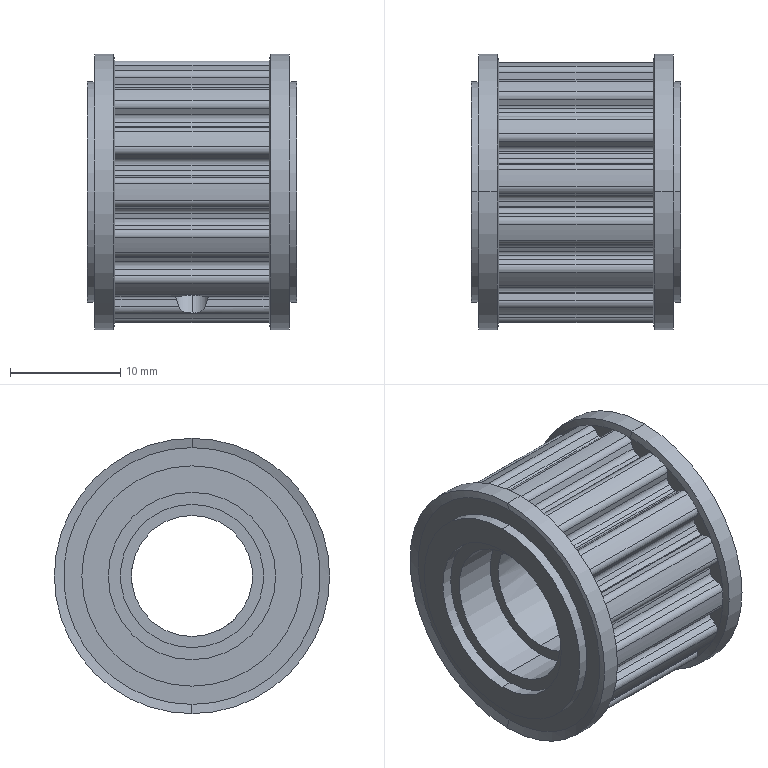Part | NX | features BREP 3 | 3 solids | 254 faces | box 19 x 25 x 25 mm | volume 5461 mm3 | cylinder 136 | plane 98 | cone 20 | commonest cylinder face diameters 1.22 x76 20.95 x17 23.75 x15 3.242 x4 4 x4 11 x4